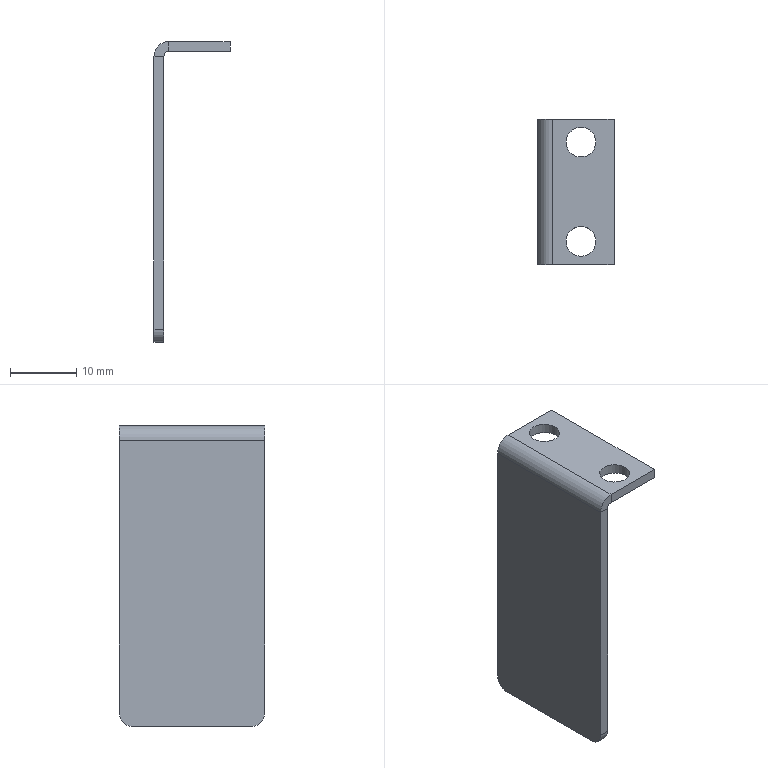Part | NX | 1 solid | 18 faces | box 11.5 x 22 x 45.5 mm | volume 1760 mm3 | plane 12 | cylinder 6 | commonest cylinder face diameters 4 x2 4.5 x2 1.473 x1 4.473 x1
STEP:
#1=CARTESIAN_POINT('',(5.,11.,-1.5));
#2=VERTEX_POINT('',#1);
#3=CARTESIAN_POINT('',(-4.263,11.,-1.5));
#4=VERTEX_POINT('',#3);
#5=CARTESIAN_POINT('',(-5.,11.,-1.5));
#6=DIRECTION('',(-1.,0.,0.));
#7=VECTOR('',#6,1000.);
#8=LINE('',#5,#7);
#9=EDGE_CURVE('',#2,#4,#8,.T.);
#10=ORIENTED_EDGE('',*,*,#9,.T.);
#11=CARTESIAN_POINT('',(-4.263,11.,0.));
#12=VERTEX_POINT('',#11);
#13=CARTESIAN_POINT('',(-4.263,11.,-1.5));
#14=DIRECTION('',(0.,0.,1.));
#15=VECTOR('',#14,1000.);
#16=LINE('',#13,#15);
#17=EDGE_CURVE('',#4,#12,#16,.T.);
#18=ORIENTED_EDGE('',*,*,#17,.T.);
#19=CARTESIAN_POINT('',(5.,11.,0.));
#20=VERTEX_POINT('',#19);
#21=CARTESIAN_POINT('',(-5.,11.,0.));
#22=DIRECTION('',(-1.,0.,0.));
#23=VECTOR('',#22,1000.);
#24=LINE('',#21,#23);
#25=EDGE_CURVE('',#20,#12,#24,.T.);
#26=ORIENTED_EDGE('',*,*,#25,.F.);
#27=CARTESIAN_POINT('',(5.,11.,-1.5));
#28=DIRECTION('',(0.,0.,1.));
#29=VECTOR('',#28,1000.);
#30=LINE('',#27,#29);
#31=EDGE_CURVE('',#2,#20,#30,.T.);
#32=ORIENTED_EDGE('',*,*,#31,.F.);
#33=EDGE_LOOP('',(#10,#18,#26,#32));
#34=FACE_BOUND('',#33,.T.);
#35=CARTESIAN_POINT('',(-5.,11.,-1.5));
#36=DIRECTION('',(0.,1.,0.));
#37=DIRECTION('',(0.,0.,1.));
#38=AXIS2_PLACEMENT_3D('',#35,#36,#37);
#39=PLANE('',#38);
#40=ADVANCED_FACE('',(#34),#39,.T.);
#41=CARTESIAN_POINT('',(-2.25,-7.5,-1.5));
#42=VERTEX_POINT('',#41);
#43=CARTESIAN_POINT('',(0.,-7.5,-1.5));
#44=DIRECTION('',(0.,0.,-1.));
#45=DIRECTION('',(-1.,0.,0.));
#46=AXIS2_PLACEMENT_3D('',#43,#44,#45);
#47=CIRCLE('',#46,2.25);
#48=EDGE_CURVE('',#42,#42,#47,.T.);
#49=ORIENTED_EDGE('',*,*,#48,.F.);
#50=EDGE_LOOP('',(#49));
#51=FACE_BOUND('',#50,.T.);
#52=CARTESIAN_POINT('',(-2.25,7.5,-1.5));
#53=VERTEX_POINT('',#52);
#54=CARTESIAN_POINT('',(0.,7.5,-1.5));
#55=DIRECTION('',(0.,0.,-1.));
#56=DIRECTION('',(-1.,0.,0.));
#57=AXIS2_PLACEMENT_3D('',#54,#55,#56);
#58=CIRCLE('',#57,2.25);
#59=EDGE_CURVE('',#53,#53,#58,.T.);
#60=ORIENTED_EDGE('',*,*,#59,.F.);
#61=EDGE_LOOP('',(#60));
#62=FACE_BOUND('',#61,.T.);
#63=CARTESIAN_POINT('',(-4.263,-11.,-1.5));
#64=VERTEX_POINT('',#63);
#65=CARTESIAN_POINT('',(5.,-11.,-1.5));
#66=VERTEX_POINT('',#65);
#67=CARTESIAN_POINT('',(-5.,-11.,-1.5));
#68=DIRECTION('',(1.,0.,0.));
#69=VECTOR('',#68,1000.);
#70=LINE('',#67,#69);
#71=EDGE_CURVE('',#64,#66,#70,.T.);
#72=ORIENTED_EDGE('',*,*,#71,.F.);
#73=CARTESIAN_POINT('',(-4.263,11.,-1.5));
#74=DIRECTION('',(0.,1.,0.));
#75=VECTOR('',#74,1000.);
#76=LINE('',#73,#75);
#77=EDGE_CURVE('',#4,#64,#76,.F.);
#78=ORIENTED_EDGE('',*,*,#77,.F.);
#79=ORIENTED_EDGE('',*,*,#9,.F.);
#80=CARTESIAN_POINT('',(5.,-11.,-1.5));
#81=DIRECTION('',(0.,1.,0.));
#82=VECTOR('',#81,1000.);
#83=LINE('',#80,#82);
#84=EDGE_CURVE('',#66,#2,#83,.T.);
#85=ORIENTED_EDGE('',*,*,#84,.F.);
#86=EDGE_LOOP('',(#72,#78,#79,#85));
#87=FACE_BOUND('',#86,.T.);
#88=CARTESIAN_POINT('',(0.,0.,-1.5));
#89=DIRECTION('',(0.,0.,-1.));
#90=DIRECTION('',(-1.,0.,0.));
#91=AXIS2_PLACEMENT_3D('',#88,#89,#90);
#92=PLANE('',#91);
#93=ADVANCED_FACE('',(#51,#62,#87),#92,.T.);
#94=CARTESIAN_POINT('',(-2.25,-7.5,0.));
#95=VERTEX_POINT('',#94);
#96=CARTESIAN_POINT('',(0.,-7.5,0.));
#97=DIRECTION('',(0.,0.,-1.));
#98=DIRECTION('',(-1.,0.,0.));
#99=AXIS2_PLACEMENT_3D('',#96,#97,#98);
#100=CIRCLE('',#99,2.25);
#101=EDGE_CURVE('',#95,#95,#100,.T.);
#102=ORIENTED_EDGE('',*,*,#101,.T.);
#103=EDGE_LOOP('',(#102));
#104=FACE_BOUND('',#103,.T.);
#105=CARTESIAN_POINT('',(-2.25,7.5,0.));
#106=VERTEX_POINT('',#105);
#107=CARTESIAN_POINT('',(0.,7.5,0.));
#108=DIRECTION('',(0.,0.,-1.));
#109=DIRECTION('',(-1.,0.,0.));
#110=AXIS2_PLACEMENT_3D('',#107,#108,#109);
#111=CIRCLE('',#110,2.25);
#112=EDGE_CURVE('',#106,#106,#111,.T.);
#113=ORIENTED_EDGE('',*,*,#112,.T.);
#114=EDGE_LOOP('',(#113));
#115=FACE_BOUND('',#114,.T.);
#116=CARTESIAN_POINT('',(-4.263,-11.,0.));
#117=VERTEX_POINT('',#116);
#118=CARTESIAN_POINT('',(-4.263,11.,0.));
#119=DIRECTION('',(0.,1.,0.));
#120=VECTOR('',#119,1000.);
#121=LINE('',#118,#120);
#122=EDGE_CURVE('',#12,#117,#121,.F.);
#123=ORIENTED_EDGE('',*,*,#122,.T.);
#124=CARTESIAN_POINT('',(5.,-11.,0.));
#125=VERTEX_POINT('',#124);
#126=CARTESIAN_POINT('',(-5.,-11.,0.));
#127=DIRECTION('',(1.,0.,0.));
#128=VECTOR('',#127,1000.);
#129=LINE('',#126,#128);
#130=EDGE_CURVE('',#117,#125,#129,.T.);
#131=ORIENTED_EDGE('',*,*,#130,.T.);
#132=CARTESIAN_POINT('',(5.,-11.,0.));
#133=DIRECTION('',(0.,1.,0.));
#134=VECTOR('',#133,1000.);
#135=LINE('',#132,#134);
#136=EDGE_CURVE('',#125,#20,#135,.T.);
#137=ORIENTED_EDGE('',*,*,#136,.T.);
#138=ORIENTED_EDGE('',*,*,#25,.T.);
#139=EDGE_LOOP('',(#123,#131,#137,#138));
#140=FACE_BOUND('',#139,.T.);
#141=CARTESIAN_POINT('',(0.,0.,0.));
#142=DIRECTION('',(0.,0.,-1.));
#143=DIRECTION('',(-1.,0.,0.));
#144=AXIS2_PLACEMENT_3D('',#141,#142,#143);
#145=PLANE('',#144);
#146=ADVANCED_FACE('',(#104,#115,#140),#145,.F.);
#147=ORIENTED_EDGE('',*,*,#136,.F.);
#148=CARTESIAN_POINT('',(5.,-11.,-1.5));
#149=DIRECTION('',(0.,0.,1.));
#150=VECTOR('',#149,1000.);
#151=LINE('',#148,#150);
#152=EDGE_CURVE('',#66,#125,#151,.T.);
#153=ORIENTED_EDGE('',*,*,#152,.F.);
#154=ORIENTED_EDGE('',*,*,#84,.T.);
#155=ORIENTED_EDGE('',*,*,#31,.T.);
#156=EDGE_LOOP('',(#147,#153,#154,#155));
#157=FACE_BOUND('',#156,.T.);
#158=CARTESIAN_POINT('',(5.,-11.,-1.5));
#159=DIRECTION('',(1.,0.,0.));
#160=DIRECTION('',(0.,0.,-1.));
#161=AXIS2_PLACEMENT_3D('',#158,#159,#160);
#162=PLANE('',#161);
#163=ADVANCED_FACE('',(#157),#162,.T.);
#164=CARTESIAN_POINT('',(-4.263,-11.,-1.5));
#165=DIRECTION('',(0.,0.,1.));
#166=VECTOR('',#165,1000.);
#167=LINE('',#164,#166);
#168=EDGE_CURVE('',#64,#117,#167,.T.);
#169=ORIENTED_EDGE('',*,*,#168,.F.);
#170=ORIENTED_EDGE('',*,*,#71,.T.);
#171=ORIENTED_EDGE('',*,*,#152,.T.);
#172=ORIENTED_EDGE('',*,*,#130,.F.);
#173=EDGE_LOOP('',(#169,#170,#171,#172));
#174=FACE_BOUND('',#173,.T.);
#175=CARTESIAN_POINT('',(-5.,-11.,-1.5));
#176=DIRECTION('',(0.,-1.,0.));
#177=DIRECTION('',(0.,0.,-1.));
#178=AXIS2_PLACEMENT_3D('',#175,#176,#177);
#179=PLANE('',#178);
#180=ADVANCED_FACE('',(#174),#179,.T.);
#181=CARTESIAN_POINT('',(-5.,-11.,-2.237));
#182=VERTEX_POINT('',#181);
#183=CARTESIAN_POINT('',(-6.5,-11.,-2.237));
#184=VERTEX_POINT('',#183);
#185=CARTESIAN_POINT('',(-5.,-11.,-2.237));
#186=DIRECTION('',(-1.,0.,0.));
#187=VECTOR('',#186,1000.);
#188=LINE('',#185,#187);
#189=EDGE_CURVE('',#182,#184,#188,.T.);
#190=ORIENTED_EDGE('',*,*,#189,.F.);
#191=CARTESIAN_POINT('',(-4.263,-11.,-2.237));
#192=DIRECTION('',(0.,1.,0.));
#193=DIRECTION('',(0.,0.,1.));
#194=AXIS2_PLACEMENT_3D('',#191,#192,#193);
#195=CIRCLE('',#194,0.7366);
#196=EDGE_CURVE('',#64,#182,#195,.F.);
#197=ORIENTED_EDGE('',*,*,#196,.F.);
#198=ORIENTED_EDGE('',*,*,#168,.T.);
#199=CARTESIAN_POINT('',(-4.263,-11.,-2.237));
#200=DIRECTION('',(0.,1.,0.));
#201=DIRECTION('',(0.,0.,1.));
#202=AXIS2_PLACEMENT_3D('',#199,#200,#201);
#203=CIRCLE('',#202,2.237);
#204=EDGE_CURVE('',#117,#184,#203,.F.);
#205=ORIENTED_EDGE('',*,*,#204,.T.);
#206=EDGE_LOOP('',(#190,#197,#198,#205));
#207=FACE_BOUND('',#206,.T.);
#208=CARTESIAN_POINT('',(-4.263,-11.,-2.237));
#209=DIRECTION('',(0.,-1.,0.));
#210=DIRECTION('',(0.,0.,-1.));
#211=AXIS2_PLACEMENT_3D('',#208,#209,#210);
#212=PLANE('',#211);
#213=ADVANCED_FACE('',(#207),#212,.T.);
#214=CARTESIAN_POINT('',(-5.,11.,-2.237));
#215=VERTEX_POINT('',#214);
#216=CARTESIAN_POINT('',(-4.263,11.,-2.237));
#217=DIRECTION('',(0.,1.,0.));
#218=DIRECTION('',(0.,0.,1.));
#219=AXIS2_PLACEMENT_3D('',#216,#217,#218);
#220=CIRCLE('',#219,0.7366);
#221=EDGE_CURVE('',#215,#4,#220,.T.);
#222=ORIENTED_EDGE('',*,*,#221,.F.);
#223=CARTESIAN_POINT('',(-6.5,11.,-2.237));
#224=VERTEX_POINT('',#223);
#225=CARTESIAN_POINT('',(-5.,11.,-2.237));
#226=DIRECTION('',(-1.,0.,0.));
#227=VECTOR('',#226,1000.);
#228=LINE('',#225,#227);
#229=EDGE_CURVE('',#215,#224,#228,.T.);
#230=ORIENTED_EDGE('',*,*,#229,.T.);
#231=CARTESIAN_POINT('',(-4.263,11.,-2.237));
#232=DIRECTION('',(0.,1.,0.));
#233=DIRECTION('',(0.,0.,1.));
#234=AXIS2_PLACEMENT_3D('',#231,#232,#233);
#235=CIRCLE('',#234,2.237);
#236=EDGE_CURVE('',#224,#12,#235,.T.);
#237=ORIENTED_EDGE('',*,*,#236,.T.);
#238=ORIENTED_EDGE('',*,*,#17,.F.);
#239=EDGE_LOOP('',(#222,#230,#237,#238));
#240=FACE_BOUND('',#239,.T.);
#241=CARTESIAN_POINT('',(-4.263,11.,-2.237));
#242=DIRECTION('',(0.,-1.,0.));
#243=DIRECTION('',(0.,0.,-1.));
#244=AXIS2_PLACEMENT_3D('',#241,#242,#243);
#245=PLANE('',#244);
#246=ADVANCED_FACE('',(#240),#245,.F.);
#247=ORIENTED_EDGE('',*,*,#122,.F.);
#248=ORIENTED_EDGE('',*,*,#236,.F.);
#249=CARTESIAN_POINT('',(-6.5,0.,-2.237));
#250=DIRECTION('',(0.,1.,0.));
#251=VECTOR('',#250,1000.);
#252=LINE('',#249,#251);
#253=EDGE_CURVE('',#184,#224,#252,.T.);
#254=ORIENTED_EDGE('',*,*,#253,.F.);
#255=ORIENTED_EDGE('',*,*,#204,.F.);
#256=EDGE_LOOP('',(#247,#248,#254,#255));
#257=FACE_BOUND('',#256,.T.);
#258=CARTESIAN_POINT('',(-4.263,11.,-2.237));
#259=DIRECTION('',(0.,1.,0.));
#260=DIRECTION('',(-1.,0.,0.));
#261=AXIS2_PLACEMENT_3D('',#258,#259,#260);
#262=CYLINDRICAL_SURFACE('',#261,2.237);
#263=ADVANCED_FACE('',(#257),#262,.T.);
#264=ORIENTED_EDGE('',*,*,#77,.T.);
#265=ORIENTED_EDGE('',*,*,#196,.T.);
#266=CARTESIAN_POINT('',(-5.,-11.,-2.237));
#267=DIRECTION('',(0.,1.,0.));
#268=VECTOR('',#267,1000.);
#269=LINE('',#266,#268);
#270=EDGE_CURVE('',#182,#215,#269,.T.);
#271=ORIENTED_EDGE('',*,*,#270,.T.);
#272=ORIENTED_EDGE('',*,*,#221,.T.);
#273=EDGE_LOOP('',(#264,#265,#271,#272));
#274=FACE_BOUND('',#273,.T.);
#275=CARTESIAN_POINT('',(-4.263,11.,-2.237));
#276=DIRECTION('',(0.,1.,0.));
#277=DIRECTION('',(-1.,0.,0.));
#278=AXIS2_PLACEMENT_3D('',#275,#276,#277);
#279=CYLINDRICAL_SURFACE('',#278,0.7366);
#280=ADVANCED_FACE('',(#274),#279,.F.);
#281=CARTESIAN_POINT('',(-5.,11.,-43.5));
#282=VERTEX_POINT('',#281);
#283=CARTESIAN_POINT('',(-5.,11.,-1.5));
#284=DIRECTION('',(0.,0.,1.));
#285=VECTOR('',#284,1000.);
#286=LINE('',#283,#285);
#287=EDGE_CURVE('',#282,#215,#286,.T.);
#288=ORIENTED_EDGE('',*,*,#287,.F.);
#289=CARTESIAN_POINT('',(-6.5,11.,-43.5));
#290=VERTEX_POINT('',#289);
#291=CARTESIAN_POINT('',(-6.5,11.,-43.5));
#292=DIRECTION('',(1.,0.,0.));
#293=VECTOR('',#292,1000.);
#294=LINE('',#291,#293);
#295=EDGE_CURVE('',#282,#290,#294,.F.);
#296=ORIENTED_EDGE('',*,*,#295,.T.);
#297=CARTESIAN_POINT('',(-6.5,11.,-1.5));
#298=DIRECTION('',(0.,0.,1.));
#299=VECTOR('',#298,1000.);
#300=LINE('',#297,#299);
#301=EDGE_CURVE('',#290,#224,#300,.T.);
#302=ORIENTED_EDGE('',*,*,#301,.T.);
#303=ORIENTED_EDGE('',*,*,#229,.F.);
#304=EDGE_LOOP('',(#288,#296,#302,#303));
#305=FACE_BOUND('',#304,.T.);
#306=CARTESIAN_POINT('',(-6.5,11.,-1.5));
#307=DIRECTION('',(0.,1.,0.));
#308=DIRECTION('',(0.,0.,1.));
#309=AXIS2_PLACEMENT_3D('',#306,#307,#308);
#310=PLANE('',#309);
#311=ADVANCED_FACE('',(#305),#310,.T.);
#312=CARTESIAN_POINT('',(-6.5,-11.,-43.5));
#313=VERTEX_POINT('',#312);
#314=CARTESIAN_POINT('',(-6.5,-11.,-45.5));
#315=DIRECTION('',(0.,0.,-1.));
#316=VECTOR('',#315,1000.);
#317=LINE('',#314,#316);
#318=EDGE_CURVE('',#184,#313,#317,.T.);
#319=ORIENTED_EDGE('',*,*,#318,.T.);
#320=CARTESIAN_POINT('',(-5.,-11.,-43.5));
#321=VERTEX_POINT('',#320);
#322=CARTESIAN_POINT('',(-6.5,-11.,-43.5));
#323=DIRECTION('',(1.,0.,0.));
#324=VECTOR('',#323,1000.);
#325=LINE('',#322,#324);
#326=EDGE_CURVE('',#313,#321,#325,.T.);
#327=ORIENTED_EDGE('',*,*,#326,.T.);
#328=CARTESIAN_POINT('',(-5.,-11.,-45.5));
#329=DIRECTION('',(0.,0.,-1.));
#330=VECTOR('',#329,1000.);
#331=LINE('',#328,#330);
#332=EDGE_CURVE('',#182,#321,#331,.T.);
#333=ORIENTED_EDGE('',*,*,#332,.F.);
#334=ORIENTED_EDGE('',*,*,#189,.T.);
#335=EDGE_LOOP('',(#319,#327,#333,#334));
#336=FACE_BOUND('',#335,.T.);
#337=CARTESIAN_POINT('',(-6.5,-11.,-45.5));
#338=DIRECTION('',(0.,-1.,0.));
#339=DIRECTION('',(0.,0.,-1.));
#340=AXIS2_PLACEMENT_3D('',#337,#338,#339);
#341=PLANE('',#340);
#342=ADVANCED_FACE('',(#336),#341,.T.);
#343=ORIENTED_EDGE('',*,*,#301,.F.);
#344=CARTESIAN_POINT('',(-6.5,9.,-45.5));
#345=VERTEX_POINT('',#344);
#346=CARTESIAN_POINT('',(-6.5,9.,-43.5));
#347=DIRECTION('',(-1.,0.,0.));
#348=DIRECTION('',(0.,0.,1.));
#349=AXIS2_PLACEMENT_3D('',#346,#347,#348);
#350=CIRCLE('',#349,2.);
#351=EDGE_CURVE('',#290,#345,#350,.T.);
#352=ORIENTED_EDGE('',*,*,#351,.T.);
#353=CARTESIAN_POINT('',(-6.5,-9.,-45.5));
#354=VERTEX_POINT('',#353);
#355=CARTESIAN_POINT('',(-6.5,11.,-45.5));
#356=DIRECTION('',(0.,1.,0.));
#357=VECTOR('',#356,1000.);
#358=LINE('',#355,#357);
#359=EDGE_CURVE('',#354,#345,#358,.T.);
#360=ORIENTED_EDGE('',*,*,#359,.F.);
#361=CARTESIAN_POINT('',(-6.5,-9.,-43.5));
#362=DIRECTION('',(-1.,0.,0.));
#363=DIRECTION('',(0.,0.,1.));
#364=AXIS2_PLACEMENT_3D('',#361,#362,#363);
#365=CIRCLE('',#364,2.);
#366=EDGE_CURVE('',#354,#313,#365,.T.);
#367=ORIENTED_EDGE('',*,*,#366,.T.);
#368=ORIENTED_EDGE('',*,*,#318,.F.);
#369=ORIENTED_EDGE('',*,*,#253,.T.);
#370=EDGE_LOOP('',(#343,#352,#360,#367,#368,#369));
#371=FACE_BOUND('',#370,.T.);
#372=CARTESIAN_POINT('',(-6.5,0.,0.));
#373=DIRECTION('',(-1.,0.,0.));
#374=DIRECTION('',(0.,0.,1.));
#375=AXIS2_PLACEMENT_3D('',#372,#373,#374);
#376=PLANE('',#375);
#377=ADVANCED_FACE('',(#371),#376,.T.);
#378=CARTESIAN_POINT('',(-5.,-9.,-45.5));
#379=VERTEX_POINT('',#378);
#380=CARTESIAN_POINT('',(-5.,9.,-45.5));
#381=VERTEX_POINT('',#380);
#382=CARTESIAN_POINT('',(-5.,11.,-45.5));
#383=DIRECTION('',(0.,1.,0.));
#384=VECTOR('',#383,1000.);
#385=LINE('',#382,#384);
#386=EDGE_CURVE('',#379,#381,#385,.T.);
#387=ORIENTED_EDGE('',*,*,#386,.T.);
#388=CARTESIAN_POINT('',(-5.,9.,-43.5));
#389=DIRECTION('',(-1.,0.,0.));
#390=DIRECTION('',(0.,0.,1.));
#391=AXIS2_PLACEMENT_3D('',#388,#389,#390);
#392=CIRCLE('',#391,2.);
#393=EDGE_CURVE('',#381,#282,#392,.F.);
#394=ORIENTED_EDGE('',*,*,#393,.T.);
#395=ORIENTED_EDGE('',*,*,#287,.T.);
#396=ORIENTED_EDGE('',*,*,#270,.F.);
#397=ORIENTED_EDGE('',*,*,#332,.T.);
#398=CARTESIAN_POINT('',(-5.,-9.,-43.5));
#399=DIRECTION('',(-1.,0.,0.));
#400=DIRECTION('',(0.,0.,1.));
#401=AXIS2_PLACEMENT_3D('',#398,#399,#400);
#402=CIRCLE('',#401,2.);
#403=EDGE_CURVE('',#321,#379,#402,.F.);
#404=ORIENTED_EDGE('',*,*,#403,.T.);
#405=EDGE_LOOP('',(#387,#394,#395,#396,#397,#404));
#406=FACE_BOUND('',#405,.T.);
#407=CARTESIAN_POINT('',(-5.,0.,0.));
#408=DIRECTION('',(-1.,0.,0.));
#409=DIRECTION('',(0.,0.,1.));
#410=AXIS2_PLACEMENT_3D('',#407,#408,#409);
#411=PLANE('',#410);
#412=ADVANCED_FACE('',(#406),#411,.F.);
#413=ORIENTED_EDGE('',*,*,#359,.T.);
#414=CARTESIAN_POINT('',(-6.5,9.,-45.5));
#415=DIRECTION('',(1.,0.,0.));
#416=VECTOR('',#415,1000.);
#417=LINE('',#414,#416);
#418=EDGE_CURVE('',#345,#381,#417,.T.);
#419=ORIENTED_EDGE('',*,*,#418,.T.);
#420=ORIENTED_EDGE('',*,*,#386,.F.);
#421=CARTESIAN_POINT('',(-6.5,-9.,-45.5));
#422=DIRECTION('',(1.,0.,0.));
#423=VECTOR('',#422,1000.);
#424=LINE('',#421,#423);
#425=EDGE_CURVE('',#379,#354,#424,.F.);
#426=ORIENTED_EDGE('',*,*,#425,.T.);
#427=EDGE_LOOP('',(#413,#419,#420,#426));
#428=FACE_BOUND('',#427,.T.);
#429=CARTESIAN_POINT('',(-6.5,11.,-45.5));
#430=DIRECTION('',(0.,0.,-1.));
#431=DIRECTION('',(-1.,0.,0.));
#432=AXIS2_PLACEMENT_3D('',#429,#430,#431);
#433=PLANE('',#432);
#434=ADVANCED_FACE('',(#428),#433,.T.);
#435=ORIENTED_EDGE('',*,*,#59,.T.);
#436=EDGE_LOOP('',(#435));
#437=FACE_BOUND('',#436,.T.);
#438=ORIENTED_EDGE('',*,*,#112,.F.);
#439=EDGE_LOOP('',(#438));
#440=FACE_BOUND('',#439,.T.);
#441=CARTESIAN_POINT('',(0.,7.5,8.5));
#442=DIRECTION('',(0.,0.,-1.));
#443=DIRECTION('',(-1.,0.,0.));
#444=AXIS2_PLACEMENT_3D('',#441,#442,#443);
#445=CYLINDRICAL_SURFACE('',#444,2.25);
#446=ADVANCED_FACE('',(#437,#440),#445,.F.);
#447=ORIENTED_EDGE('',*,*,#48,.T.);
#448=EDGE_LOOP('',(#447));
#449=FACE_BOUND('',#448,.T.);
#450=ORIENTED_EDGE('',*,*,#101,.F.);
#451=EDGE_LOOP('',(#450));
#452=FACE_BOUND('',#451,.T.);
#453=CARTESIAN_POINT('',(0.,-7.5,8.5));
#454=DIRECTION('',(0.,0.,-1.));
#455=DIRECTION('',(-1.,0.,0.));
#456=AXIS2_PLACEMENT_3D('',#453,#454,#455);
#457=CYLINDRICAL_SURFACE('',#456,2.25);
#458=ADVANCED_FACE('',(#449,#452),#457,.F.);
#459=ORIENTED_EDGE('',*,*,#351,.F.);
#460=ORIENTED_EDGE('',*,*,#295,.F.);
#461=ORIENTED_EDGE('',*,*,#393,.F.);
#462=ORIENTED_EDGE('',*,*,#418,.F.);
#463=EDGE_LOOP('',(#459,#460,#461,#462));
#464=FACE_BOUND('',#463,.T.);
#465=CARTESIAN_POINT('',(-6.5,9.,-43.5));
#466=DIRECTION('',(1.,0.,0.));
#467=DIRECTION('',(0.,0.,-1.));
#468=AXIS2_PLACEMENT_3D('',#465,#466,#467);
#469=CYLINDRICAL_SURFACE('',#468,2.);
#470=ADVANCED_FACE('',(#464),#469,.T.);
#471=ORIENTED_EDGE('',*,*,#366,.F.);
#472=ORIENTED_EDGE('',*,*,#425,.F.);
#473=ORIENTED_EDGE('',*,*,#403,.F.);
#474=ORIENTED_EDGE('',*,*,#326,.F.);
#475=EDGE_LOOP('',(#471,#472,#473,#474));
#476=FACE_BOUND('',#475,.T.);
#477=CARTESIAN_POINT('',(-6.5,-9.,-43.5));
#478=DIRECTION('',(1.,0.,0.));
#479=DIRECTION('',(0.,0.,-1.));
#480=AXIS2_PLACEMENT_3D('',#477,#478,#479);
#481=CYLINDRICAL_SURFACE('',#480,2.);
#482=ADVANCED_FACE('',(#476),#481,.T.);
#483=CLOSED_SHELL('',(#40,#93,#146,#163,#180,#213,#246,#263,#280,#311,#342,#377,#412,#434,#446,#458,#470,#482));
#484=MANIFOLD_SOLID_BREP('',#483);
#485=(LENGTH_UNIT()NAMED_UNIT(*)SI_UNIT(.MILLI.,.METRE.));
#486=UNCERTAINTY_MEASURE_WITH_UNIT(LENGTH_MEASURE(0.00001),#485,'','');
#487=(NAMED_UNIT(*)PLANE_ANGLE_UNIT()SI_UNIT($,.RADIAN.));
#488=(NAMED_UNIT(*)SI_UNIT($,.STERADIAN.)SOLID_ANGLE_UNIT());
#489=(GEOMETRIC_REPRESENTATION_CONTEXT(3)GLOBAL_UNCERTAINTY_ASSIGNED_CONTEXT((#486))GLOBAL_UNIT_ASSIGNED_CONTEXT((#485,#487,#488))REPRESENTATION_CONTEXT('',''));
#490=ADVANCED_BREP_SHAPE_REPRESENTATION('',(#484),#489);